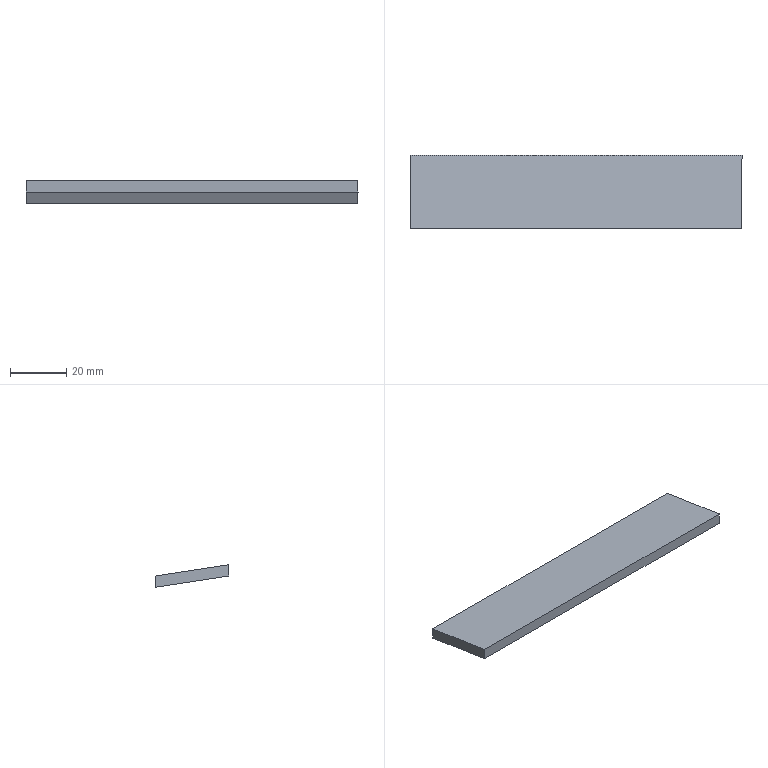Part | SolidWorks | features Blend 1, BlendCut 1, ICE 1 | 1 solid | 6 faces | box 118 x 26 x 8 mm | volume 12272 mm3 | plane 4 | spline 2
STEP:
#1=CARTESIAN_POINT('',(-941.,-26.,-1101.));
#2=VERTEX_POINT('',#1);
#3=CARTESIAN_POINT('',(-941.,-26.,-1105.));
#4=VERTEX_POINT('',#3);
#5=CARTESIAN_POINT('',(-941.,-26.,991.));
#6=DIRECTION('',(0.,0.,-1.));
#7=VECTOR('',#6,1000.);
#8=LINE('',#5,#7);
#9=EDGE_CURVE('',#2,#4,#8,.T.);
#10=ORIENTED_EDGE('',*,*,#9,.F.);
#11=CARTESIAN_POINT('',(-1059.,-26.,-1101.));
#12=VERTEX_POINT('',#11);
#13=CARTESIAN_POINT('',(0.,-26.,-1101.));
#14=DIRECTION('',(-1.,0.,0.));
#15=VECTOR('',#14,1000.);
#16=LINE('',#13,#15);
#17=EDGE_CURVE('',#2,#12,#16,.T.);
#18=ORIENTED_EDGE('',*,*,#17,.T.);
#19=CARTESIAN_POINT('',(-1059.,-26.,-1105.));
#20=VERTEX_POINT('',#19);
#21=CARTESIAN_POINT('',(-1059.,-26.,991.));
#22=DIRECTION('',(0.,0.,1.));
#23=VECTOR('',#22,1000.);
#24=LINE('',#21,#23);
#25=EDGE_CURVE('',#20,#12,#24,.T.);
#26=ORIENTED_EDGE('',*,*,#25,.F.);
#27=CARTESIAN_POINT('',(0.,-26.,-1105.));
#28=DIRECTION('',(1.,0.,0.));
#29=VECTOR('',#28,1000.);
#30=LINE('',#27,#29);
#31=EDGE_CURVE('',#20,#4,#30,.T.);
#32=ORIENTED_EDGE('',*,*,#31,.T.);
#33=EDGE_LOOP('',(#10,#18,#26,#32));
#34=FACE_OUTER_BOUND('',#33,.T.);
#35=CARTESIAN_POINT('',(-1191.,-26.,991.));
#36=DIRECTION('',(0.,1.,0.));
#37=DIRECTION('',(0.,0.,1.));
#38=AXIS2_PLACEMENT_3D('',#35,#36,#37);
#39=PLANE('',#38);
#40=ADVANCED_FACE('',(#34),#39,.F.);
#41=CARTESIAN_POINT('',(-941.,0.,-1105.));
#42=VERTEX_POINT('',#41);
#43=CARTESIAN_POINT('',(-941.,0.,-1109.));
#44=VERTEX_POINT('',#43);
#45=CARTESIAN_POINT('',(-941.,0.,-1109.));
#46=DIRECTION('',(0.,0.,-1.));
#47=VECTOR('',#46,1000.);
#48=LINE('',#45,#47);
#49=EDGE_CURVE('',#42,#44,#48,.T.);
#50=ORIENTED_EDGE('',*,*,#49,.T.);
#51=CARTESIAN_POINT('',(-1059.,0.,-1109.));
#52=VERTEX_POINT('',#51);
#53=CARTESIAN_POINT('',(0.,0.,-1109.));
#54=DIRECTION('',(-1.,0.,0.));
#55=VECTOR('',#54,1000.);
#56=LINE('',#53,#55);
#57=EDGE_CURVE('',#44,#52,#56,.T.);
#58=ORIENTED_EDGE('',*,*,#57,.T.);
#59=CARTESIAN_POINT('',(-1059.,0.,-1105.));
#60=VERTEX_POINT('',#59);
#61=CARTESIAN_POINT('',(-1059.,0.,-1109.));
#62=DIRECTION('',(0.,0.,1.));
#63=VECTOR('',#62,1000.);
#64=LINE('',#61,#63);
#65=EDGE_CURVE('',#52,#60,#64,.T.);
#66=ORIENTED_EDGE('',*,*,#65,.T.);
#67=CARTESIAN_POINT('',(0.,0.,-1105.));
#68=DIRECTION('',(-1.,0.,0.));
#69=VECTOR('',#68,1000.);
#70=LINE('',#67,#69);
#71=EDGE_CURVE('',#42,#60,#70,.T.);
#72=ORIENTED_EDGE('',*,*,#71,.F.);
#73=EDGE_LOOP('',(#50,#58,#66,#72));
#74=FACE_OUTER_BOUND('',#73,.T.);
#75=CARTESIAN_POINT('',(-1191.,0.,991.));
#76=DIRECTION('',(0.,-1.,0.));
#77=DIRECTION('',(0.,0.,-1.));
#78=AXIS2_PLACEMENT_3D('',#75,#76,#77);
#79=PLANE('',#78);
#80=ADVANCED_FACE('',(#74),#79,.F.);
#81=ORIENTED_EDGE('',*,*,#57,.F.);
#82=CARTESIAN_POINT('',(-941.,0.,-1109.));
#83=CARTESIAN_POINT('',(-941.,-2.168,-1108.666));
#84=CARTESIAN_POINT('',(-941.,-4.336,-1108.333));
#85=CARTESIAN_POINT('',(-941.,-6.504,-1107.999));
#86=CARTESIAN_POINT('',(-941.,-8.672,-1107.666));
#87=CARTESIAN_POINT('',(-941.,-10.84,-1107.332));
#88=CARTESIAN_POINT('',(-941.,-13.008,-1106.999));
#89=CARTESIAN_POINT('',(-941.,-17.338,-1106.333));
#90=CARTESIAN_POINT('',(-941.,-21.669,-1105.666));
#91=CARTESIAN_POINT('',(-941.,-26.,-1105.));
#92=B_SPLINE_CURVE_WITH_KNOTS('',3,(#82,#83,#84,#85,#86,#87,#88,#89,#90,#91),.UNSPECIFIED.,.F.,.F.,(4,3,3,4),(0.,0.00658,0.01316,0.02631),.UNSPECIFIED.);
#93=EDGE_CURVE('',#44,#4,#92,.T.);
#94=ORIENTED_EDGE('',*,*,#93,.T.);
#95=ORIENTED_EDGE('',*,*,#31,.F.);
#96=CARTESIAN_POINT('',(-1059.,-26.,-1105.));
#97=CARTESIAN_POINT('',(-1059.,-23.832,-1105.334));
#98=CARTESIAN_POINT('',(-1059.,-21.664,-1105.667));
#99=CARTESIAN_POINT('',(-1059.,-19.496,-1106.001));
#100=CARTESIAN_POINT('',(-1059.,-17.328,-1106.334));
#101=CARTESIAN_POINT('',(-1059.,-15.16,-1106.668));
#102=CARTESIAN_POINT('',(-1059.,-12.992,-1107.001));
#103=CARTESIAN_POINT('',(-1059.,-8.662,-1107.667));
#104=CARTESIAN_POINT('',(-1059.,-4.331,-1108.334));
#105=CARTESIAN_POINT('',(-1059.,0.,-1109.));
#106=B_SPLINE_CURVE_WITH_KNOTS('',3,(#96,#97,#98,#99,#100,#101,#102,#103,#104,#105),.UNSPECIFIED.,.F.,.F.,(4,3,3,4),(0.,0.00658,0.01316,0.02631),.UNSPECIFIED.);
#107=EDGE_CURVE('',#20,#52,#106,.T.);
#108=ORIENTED_EDGE('',*,*,#107,.T.);
#109=EDGE_LOOP('',(#81,#94,#95,#108));
#110=FACE_OUTER_BOUND('',#109,.T.);
#111=CARTESIAN_POINT('',(-1309.,0.,991.));
#112=CARTESIAN_POINT('',(-1305.,-26.,991.));
#113=CARTESIAN_POINT('',(-1309.,0.,825.593));
#114=CARTESIAN_POINT('',(-1305.,-26.,826.073));
#115=CARTESIAN_POINT('',(-1309.,0.,495.141));
#116=CARTESIAN_POINT('',(-1305.,-26.,495.86));
#117=CARTESIAN_POINT('',(-1309.,0.,0.));
#118=CARTESIAN_POINT('',(-1305.,-26.,0.));
#119=CARTESIAN_POINT('',(-1309.,0.,-495.141));
#120=CARTESIAN_POINT('',(-1305.,-26.,-495.86));
#121=CARTESIAN_POINT('',(-1309.,0.,-825.593));
#122=CARTESIAN_POINT('',(-1305.,-26.,-826.073));
#123=CARTESIAN_POINT('',(-1309.,0.,-998.603));
#124=CARTESIAN_POINT('',(-1305.,-26.,-998.581));
#125=CARTESIAN_POINT('',(-1307.525,0.,-1013.896));
#126=CARTESIAN_POINT('',(-1303.485,-26.,-1013.65));
#127=CARTESIAN_POINT('',(-1300.841,0.,-1036.165));
#128=CARTESIAN_POINT('',(-1296.885,-26.,-1035.179));
#129=CARTESIAN_POINT('',(-1289.866,0.,-1056.819));
#130=CARTESIAN_POINT('',(-1286.285,-26.,-1054.896));
#131=CARTESIAN_POINT('',(-1275.,0.,-1074.971));
#132=CARTESIAN_POINT('',(-1272.108,-26.,-1072.135));
#133=CARTESIAN_POINT('',(-1256.851,0.,-1089.845));
#134=CARTESIAN_POINT('',(-1254.866,-26.,-1086.305));
#135=CARTESIAN_POINT('',(-1236.193,0.,-1100.83));
#136=CARTESIAN_POINT('',(-1235.152,-26.,-1096.895));
#137=CARTESIAN_POINT('',(-1213.914,0.,-1107.523));
#138=CARTESIAN_POINT('',(-1213.633,-26.,-1103.487));
#139=CARTESIAN_POINT('',(-1198.609,0.,-1109.));
#140=CARTESIAN_POINT('',(-1198.575,-26.,-1105.));
#141=CARTESIAN_POINT('',(-1091.523,0.,-1109.));
#142=CARTESIAN_POINT('',(-1091.977,-26.,-1105.));
#143=CARTESIAN_POINT('',(-892.796,0.,-1109.));
#144=CARTESIAN_POINT('',(-893.704,-26.,-1105.));
#145=CARTESIAN_POINT('',(-595.132,0.,-1109.));
#146=CARTESIAN_POINT('',(-595.87,-26.,-1105.));
#147=CARTESIAN_POINT('',(-297.637,0.,-1109.));
#148=CARTESIAN_POINT('',(-297.864,-26.,-1105.));
#149=CARTESIAN_POINT('',(-99.25,0.,-1109.));
#150=CARTESIAN_POINT('',(-99.25,-26.,-1105.));
#151=CARTESIAN_POINT('',(99.25,0.,-1109.));
#152=CARTESIAN_POINT('',(99.25,-26.,-1105.));
#153=CARTESIAN_POINT('',(297.637,0.,-1109.));
#154=CARTESIAN_POINT('',(297.864,-26.,-1105.));
#155=CARTESIAN_POINT('',(595.132,0.,-1109.));
#156=CARTESIAN_POINT('',(595.87,-26.,-1105.));
#157=CARTESIAN_POINT('',(892.796,0.,-1109.));
#158=CARTESIAN_POINT('',(893.704,-26.,-1105.));
#159=CARTESIAN_POINT('',(1091.523,0.,-1109.));
#160=CARTESIAN_POINT('',(1091.977,-26.,-1105.));
#161=CARTESIAN_POINT('',(1198.609,0.,-1109.));
#162=CARTESIAN_POINT('',(1198.575,-26.,-1105.));
#163=CARTESIAN_POINT('',(1213.914,0.,-1107.523));
#164=CARTESIAN_POINT('',(1213.633,-26.,-1103.487));
#165=CARTESIAN_POINT('',(1236.193,0.,-1100.83));
#166=CARTESIAN_POINT('',(1235.152,-26.,-1096.895));
#167=CARTESIAN_POINT('',(1256.851,0.,-1089.845));
#168=CARTESIAN_POINT('',(1254.866,-26.,-1086.305));
#169=CARTESIAN_POINT('',(1275.,0.,-1074.971));
#170=CARTESIAN_POINT('',(1272.108,-26.,-1072.135));
#171=CARTESIAN_POINT('',(1289.866,0.,-1056.819));
#172=CARTESIAN_POINT('',(1286.285,-26.,-1054.896));
#173=CARTESIAN_POINT('',(1300.841,0.,-1036.165));
#174=CARTESIAN_POINT('',(1296.885,-26.,-1035.179));
#175=CARTESIAN_POINT('',(1307.525,0.,-1013.896));
#176=CARTESIAN_POINT('',(1303.485,-26.,-1013.65));
#177=CARTESIAN_POINT('',(1309.,0.,-998.603));
#178=CARTESIAN_POINT('',(1305.,-26.,-998.581));
#179=CARTESIAN_POINT('',(1309.,0.,-825.593));
#180=CARTESIAN_POINT('',(1305.,-26.,-826.073));
#181=CARTESIAN_POINT('',(1309.,0.,-495.141));
#182=CARTESIAN_POINT('',(1305.,-26.,-495.86));
#183=CARTESIAN_POINT('',(1309.,0.,0.));
#184=CARTESIAN_POINT('',(1305.,-26.,0.));
#185=CARTESIAN_POINT('',(1309.,0.,495.141));
#186=CARTESIAN_POINT('',(1305.,-26.,495.86));
#187=CARTESIAN_POINT('',(1309.,0.,825.593));
#188=CARTESIAN_POINT('',(1305.,-26.,826.073));
#189=CARTESIAN_POINT('',(1309.,0.,998.603));
#190=CARTESIAN_POINT('',(1305.,-26.,998.581));
#191=CARTESIAN_POINT('',(1307.525,0.,1013.896));
#192=CARTESIAN_POINT('',(1303.485,-26.,1013.65));
#193=CARTESIAN_POINT('',(1300.841,0.,1036.165));
#194=CARTESIAN_POINT('',(1296.885,-26.,1035.179));
#195=CARTESIAN_POINT('',(1289.866,0.,1056.819));
#196=CARTESIAN_POINT('',(1286.285,-26.,1054.896));
#197=CARTESIAN_POINT('',(1275.,0.,1074.971));
#198=CARTESIAN_POINT('',(1272.108,-26.,1072.135));
#199=CARTESIAN_POINT('',(1256.851,0.,1089.845));
#200=CARTESIAN_POINT('',(1254.866,-26.,1086.305));
#201=CARTESIAN_POINT('',(1236.193,0.,1100.83));
#202=CARTESIAN_POINT('',(1235.152,-26.,1096.895));
#203=CARTESIAN_POINT('',(1213.914,0.,1107.523));
#204=CARTESIAN_POINT('',(1213.633,-26.,1103.487));
#205=CARTESIAN_POINT('',(1198.609,0.,1109.));
#206=CARTESIAN_POINT('',(1198.575,-26.,1105.));
#207=CARTESIAN_POINT('',(1091.523,0.,1109.));
#208=CARTESIAN_POINT('',(1091.977,-26.,1105.));
#209=CARTESIAN_POINT('',(892.796,0.,1109.));
#210=CARTESIAN_POINT('',(893.704,-26.,1105.));
#211=CARTESIAN_POINT('',(595.132,0.,1109.));
#212=CARTESIAN_POINT('',(595.87,-26.,1105.));
#213=CARTESIAN_POINT('',(297.637,0.,1109.));
#214=CARTESIAN_POINT('',(297.864,-26.,1105.));
#215=CARTESIAN_POINT('',(99.25,0.,1109.));
#216=CARTESIAN_POINT('',(99.25,-26.,1105.));
#217=CARTESIAN_POINT('',(-99.25,0.,1109.));
#218=CARTESIAN_POINT('',(-99.25,-26.,1105.));
#219=CARTESIAN_POINT('',(-297.637,0.,1109.));
#220=CARTESIAN_POINT('',(-297.864,-26.,1105.));
#221=CARTESIAN_POINT('',(-595.132,0.,1109.));
#222=CARTESIAN_POINT('',(-595.87,-26.,1105.));
#223=CARTESIAN_POINT('',(-892.796,0.,1109.));
#224=CARTESIAN_POINT('',(-893.704,-26.,1105.));
#225=CARTESIAN_POINT('',(-1091.523,0.,1109.));
#226=CARTESIAN_POINT('',(-1091.977,-26.,1105.));
#227=CARTESIAN_POINT('',(-1198.609,0.,1109.));
#228=CARTESIAN_POINT('',(-1198.575,-26.,1105.));
#229=CARTESIAN_POINT('',(-1213.914,0.,1107.523));
#230=CARTESIAN_POINT('',(-1213.633,-26.,1103.487));
#231=CARTESIAN_POINT('',(-1236.193,0.,1100.83));
#232=CARTESIAN_POINT('',(-1235.152,-26.,1096.895));
#233=CARTESIAN_POINT('',(-1256.851,0.,1089.845));
#234=CARTESIAN_POINT('',(-1254.866,-26.,1086.305));
#235=CARTESIAN_POINT('',(-1275.,0.,1074.971));
#236=CARTESIAN_POINT('',(-1272.108,-26.,1072.135));
#237=CARTESIAN_POINT('',(-1289.866,0.,1056.819));
#238=CARTESIAN_POINT('',(-1286.285,-26.,1054.896));
#239=CARTESIAN_POINT('',(-1300.841,0.,1036.165));
#240=CARTESIAN_POINT('',(-1296.885,-26.,1035.179));
#241=CARTESIAN_POINT('',(-1307.525,0.,1013.896));
#242=CARTESIAN_POINT('',(-1303.485,-26.,1013.65));
#243=CARTESIAN_POINT('',(-1309.,0.,998.603));
#244=CARTESIAN_POINT('',(-1305.,-26.,998.581));
#245=CARTESIAN_POINT('',(-1309.,0.,991.));
#246=CARTESIAN_POINT('',(-1305.,-26.,991.));
#247=B_SPLINE_SURFACE_WITH_KNOTS('',3,1,((#111,#112),(#113,#114),(#115,#116),(#117,#118),(#119,#120),(#121,#122),(#123,#124),(#125,#126),(#127,#128),(#129,#130),(#131,#132),(#133,#134),(#135,#136),(#137,#138),(#139,#140),(#141,#142),(#143,#144),(#145,#146),(#147,#148),(#149,#150),(#151,#152),(#153,#154),(#155,#156),(#157,#158),(#159,#160),(#161,#162),(#163,#164),(#165,#166),(#167,#168),(#169,#170),(#171,#172),(#173,#174),(#175,#176),(#177,#178),(#179,#180),(#181,#182),(#183,#184),(#185,#186),(#187,#188),(#189,#190),(#191,#192),(#193,#194),(#195,#196),(#197,#198),(#199,#200),(#201,#202),(#203,#204),(#205,#206),(#207,#208),(#209,#210),(#211,#212),(#213,#214),(#215,#216),(#217,#218),(#219,#220),(#221,#222),(#223,#224),(#225,#226),(#227,#228),(#229,#230),(#231,#232),(#233,#234),(#235,#236),(#237,#238),(#239,#240),(#241,#242),(#243,#244),(#245,#246)),.UNSPECIFIED.,.T.,.F.,.F.,(4,1,1,1,2,1,1,1,1,1,1,1,2,1,1,1,2,1,1,1,2,1,1,1,1,1,1,1,2,1,1,1,2,1,1,1,1,1,1,1,2,1,1,1,2,1,1,1,2,1,1,1,1,1,1,1,4),(2,2),(0.,0.0524,0.1048,0.1572,0.2096,0.212,0.2144,0.2168,0.2192,0.2216,0.224,0.2264,0.2289,0.2603,0.2918,0.3233,0.3548,0.3863,0.4178,0.4492,0.4807,0.4831,0.4855,0.488,0.4904,0.4928,0.4952,0.4976,0.5,0.5524,0.6048,0.6572,0.7096,0.712,0.7144,0.7168,0.7192,0.7216,0.724,0.7264,0.7289,0.7603,0.7918,0.8233,0.8548,0.8863,0.9178,0.9492,0.9807,0.9831,0.9855,0.988,0.9904,0.9928,0.9952,0.9976,1.),(0.,1.),.UNSPECIFIED.);
#248=ADVANCED_FACE('',(#110),#247,.T.);
#249=CARTESIAN_POINT('',(-941.,0.,-1105.));
#250=CARTESIAN_POINT('',(-941.,-2.168,-1104.666));
#251=CARTESIAN_POINT('',(-941.,-4.336,-1104.333));
#252=CARTESIAN_POINT('',(-941.,-6.504,-1103.999));
#253=CARTESIAN_POINT('',(-941.,-8.672,-1103.666));
#254=CARTESIAN_POINT('',(-941.,-10.84,-1103.332));
#255=CARTESIAN_POINT('',(-941.,-13.008,-1102.999));
#256=CARTESIAN_POINT('',(-941.,-17.339,-1102.333));
#257=CARTESIAN_POINT('',(-941.,-21.669,-1101.666));
#258=CARTESIAN_POINT('',(-941.,-26.,-1101.));
#259=B_SPLINE_CURVE_WITH_KNOTS('',3,(#249,#250,#251,#252,#253,#254,#255,#256,#257,#258),.UNSPECIFIED.,.F.,.F.,(4,3,3,4),(0.,0.00658,0.01316,0.02631),.UNSPECIFIED.);
#260=EDGE_CURVE('',#42,#2,#259,.T.);
#261=ORIENTED_EDGE('',*,*,#260,.F.);
#262=ORIENTED_EDGE('',*,*,#71,.T.);
#263=CARTESIAN_POINT('',(-1059.,-26.,-1101.));
#264=CARTESIAN_POINT('',(-1059.,-23.832,-1101.334));
#265=CARTESIAN_POINT('',(-1059.,-21.664,-1101.667));
#266=CARTESIAN_POINT('',(-1059.,-19.496,-1102.001));
#267=CARTESIAN_POINT('',(-1059.,-17.328,-1102.334));
#268=CARTESIAN_POINT('',(-1059.,-15.16,-1102.668));
#269=CARTESIAN_POINT('',(-1059.,-12.992,-1103.001));
#270=CARTESIAN_POINT('',(-1059.,-8.661,-1103.667));
#271=CARTESIAN_POINT('',(-1059.,-4.331,-1104.334));
#272=CARTESIAN_POINT('',(-1059.,0.,-1105.));
#273=B_SPLINE_CURVE_WITH_KNOTS('',3,(#263,#264,#265,#266,#267,#268,#269,#270,#271,#272),.UNSPECIFIED.,.F.,.F.,(4,3,3,4),(0.,0.00658,0.01316,0.02631),.UNSPECIFIED.);
#274=EDGE_CURVE('',#12,#60,#273,.T.);
#275=ORIENTED_EDGE('',*,*,#274,.F.);
#276=ORIENTED_EDGE('',*,*,#17,.F.);
#277=EDGE_LOOP('',(#261,#262,#275,#276));
#278=FACE_OUTER_BOUND('',#277,.T.);
#279=CARTESIAN_POINT('',(-1305.,0.,991.));
#280=CARTESIAN_POINT('',(-1301.,-26.,991.));
#281=CARTESIAN_POINT('',(-1305.,0.,825.593));
#282=CARTESIAN_POINT('',(-1301.,-26.,826.073));
#283=CARTESIAN_POINT('',(-1305.,0.,495.14));
#284=CARTESIAN_POINT('',(-1301.,-26.,495.861));
#285=CARTESIAN_POINT('',(-1305.,0.,0.));
#286=CARTESIAN_POINT('',(-1301.,-26.,0.));
#287=CARTESIAN_POINT('',(-1305.,0.,-495.14));
#288=CARTESIAN_POINT('',(-1301.,-26.,-495.861));
#289=CARTESIAN_POINT('',(-1305.,0.,-825.593));
#290=CARTESIAN_POINT('',(-1301.,-26.,-826.073));
#291=CARTESIAN_POINT('',(-1305.,0.,-998.341));
#292=CARTESIAN_POINT('',(-1301.,-26.,-998.32));
#293=CARTESIAN_POINT('',(-1303.577,0.,-1013.11));
#294=CARTESIAN_POINT('',(-1299.536,-26.,-1012.866));
#295=CARTESIAN_POINT('',(-1297.122,0.,-1034.623));
#296=CARTESIAN_POINT('',(-1293.165,-26.,-1033.638));
#297=CARTESIAN_POINT('',(-1286.518,0.,-1054.583));
#298=CARTESIAN_POINT('',(-1282.938,-26.,-1052.659));
#299=CARTESIAN_POINT('',(-1272.153,0.,-1072.125));
#300=CARTESIAN_POINT('',(-1269.262,-26.,-1069.288));
#301=CARTESIAN_POINT('',(-1254.614,0.,-1086.498));
#302=CARTESIAN_POINT('',(-1252.63,-26.,-1082.957));
#303=CARTESIAN_POINT('',(-1234.651,0.,-1097.111));
#304=CARTESIAN_POINT('',(-1233.612,-26.,-1093.175));
#305=CARTESIAN_POINT('',(-1213.127,0.,-1103.574));
#306=CARTESIAN_POINT('',(-1212.849,-26.,-1099.539));
#307=CARTESIAN_POINT('',(-1198.347,0.,-1105.));
#308=CARTESIAN_POINT('',(-1198.313,-26.,-1101.));
#309=CARTESIAN_POINT('',(-1091.522,0.,-1105.));
#310=CARTESIAN_POINT('',(-1091.978,-26.,-1101.));
#311=CARTESIAN_POINT('',(-892.794,0.,-1105.));
#312=CARTESIAN_POINT('',(-893.707,-26.,-1101.));
#313=CARTESIAN_POINT('',(-595.13,0.,-1105.));
#314=CARTESIAN_POINT('',(-595.871,-26.,-1101.));
#315=CARTESIAN_POINT('',(-297.636,0.,-1105.));
#316=CARTESIAN_POINT('',(-297.864,-26.,-1101.));
#317=CARTESIAN_POINT('',(-99.25,0.,-1105.));
#318=CARTESIAN_POINT('',(-99.25,-26.,-1101.));
#319=CARTESIAN_POINT('',(99.25,0.,-1105.));
#320=CARTESIAN_POINT('',(99.25,-26.,-1101.));
#321=CARTESIAN_POINT('',(297.636,0.,-1105.));
#322=CARTESIAN_POINT('',(297.864,-26.,-1101.));
#323=CARTESIAN_POINT('',(595.13,0.,-1105.));
#324=CARTESIAN_POINT('',(595.871,-26.,-1101.));
#325=CARTESIAN_POINT('',(892.794,0.,-1105.));
#326=CARTESIAN_POINT('',(893.707,-26.,-1101.));
#327=CARTESIAN_POINT('',(1091.522,0.,-1105.));
#328=CARTESIAN_POINT('',(1091.978,-26.,-1101.));
#329=CARTESIAN_POINT('',(1198.347,0.,-1105.));
#330=CARTESIAN_POINT('',(1198.313,-26.,-1101.));
#331=CARTESIAN_POINT('',(1213.127,0.,-1103.574));
#332=CARTESIAN_POINT('',(1212.849,-26.,-1099.539));
#333=CARTESIAN_POINT('',(1234.651,0.,-1097.111));
#334=CARTESIAN_POINT('',(1233.612,-26.,-1093.175));
#335=CARTESIAN_POINT('',(1254.614,0.,-1086.498));
#336=CARTESIAN_POINT('',(1252.63,-26.,-1082.957));
#337=CARTESIAN_POINT('',(1272.153,0.,-1072.125));
#338=CARTESIAN_POINT('',(1269.262,-26.,-1069.288));
#339=CARTESIAN_POINT('',(1286.518,0.,-1054.583));
#340=CARTESIAN_POINT('',(1282.938,-26.,-1052.659));
#341=CARTESIAN_POINT('',(1297.122,0.,-1034.623));
#342=CARTESIAN_POINT('',(1293.165,-26.,-1033.638));
#343=CARTESIAN_POINT('',(1303.577,0.,-1013.11));
#344=CARTESIAN_POINT('',(1299.536,-26.,-1012.866));
#345=CARTESIAN_POINT('',(1305.,0.,-998.341));
#346=CARTESIAN_POINT('',(1301.,-26.,-998.32));
#347=CARTESIAN_POINT('',(1305.,0.,-825.593));
#348=CARTESIAN_POINT('',(1301.,-26.,-826.073));
#349=CARTESIAN_POINT('',(1305.,0.,-495.14));
#350=CARTESIAN_POINT('',(1301.,-26.,-495.861));
#351=CARTESIAN_POINT('',(1305.,0.,0.));
#352=CARTESIAN_POINT('',(1301.,-26.,0.));
#353=CARTESIAN_POINT('',(1305.,0.,495.14));
#354=CARTESIAN_POINT('',(1301.,-26.,495.861));
#355=CARTESIAN_POINT('',(1305.,0.,825.593));
#356=CARTESIAN_POINT('',(1301.,-26.,826.073));
#357=CARTESIAN_POINT('',(1305.,0.,998.341));
#358=CARTESIAN_POINT('',(1301.,-26.,998.32));
#359=CARTESIAN_POINT('',(1303.577,0.,1013.11));
#360=CARTESIAN_POINT('',(1299.536,-26.,1012.866));
#361=CARTESIAN_POINT('',(1297.122,0.,1034.623));
#362=CARTESIAN_POINT('',(1293.165,-26.,1033.638));
#363=CARTESIAN_POINT('',(1286.518,0.,1054.583));
#364=CARTESIAN_POINT('',(1282.938,-26.,1052.659));
#365=CARTESIAN_POINT('',(1272.153,0.,1072.125));
#366=CARTESIAN_POINT('',(1269.262,-26.,1069.288));
#367=CARTESIAN_POINT('',(1254.614,0.,1086.498));
#368=CARTESIAN_POINT('',(1252.63,-26.,1082.957));
#369=CARTESIAN_POINT('',(1234.651,0.,1097.111));
#370=CARTESIAN_POINT('',(1233.612,-26.,1093.175));
#371=CARTESIAN_POINT('',(1213.127,0.,1103.574));
#372=CARTESIAN_POINT('',(1212.849,-26.,1099.539));
#373=CARTESIAN_POINT('',(1198.347,0.,1105.));
#374=CARTESIAN_POINT('',(1198.313,-26.,1101.));
#375=CARTESIAN_POINT('',(1091.522,0.,1105.));
#376=CARTESIAN_POINT('',(1091.978,-26.,1101.));
#377=CARTESIAN_POINT('',(892.794,0.,1105.));
#378=CARTESIAN_POINT('',(893.707,-26.,1101.));
#379=CARTESIAN_POINT('',(595.13,0.,1105.));
#380=CARTESIAN_POINT('',(595.871,-26.,1101.));
#381=CARTESIAN_POINT('',(297.636,0.,1105.));
#382=CARTESIAN_POINT('',(297.864,-26.,1101.));
#383=CARTESIAN_POINT('',(99.25,0.,1105.));
#384=CARTESIAN_POINT('',(99.25,-26.,1101.));
#385=CARTESIAN_POINT('',(-99.25,0.,1105.));
#386=CARTESIAN_POINT('',(-99.25,-26.,1101.));
#387=CARTESIAN_POINT('',(-297.636,0.,1105.));
#388=CARTESIAN_POINT('',(-297.864,-26.,1101.));
#389=CARTESIAN_POINT('',(-595.13,0.,1105.));
#390=CARTESIAN_POINT('',(-595.871,-26.,1101.));
#391=CARTESIAN_POINT('',(-892.794,0.,1105.));
#392=CARTESIAN_POINT('',(-893.707,-26.,1101.));
#393=CARTESIAN_POINT('',(-1091.522,0.,1105.));
#394=CARTESIAN_POINT('',(-1091.978,-26.,1101.));
#395=CARTESIAN_POINT('',(-1198.347,0.,1105.));
#396=CARTESIAN_POINT('',(-1198.313,-26.,1101.));
#397=CARTESIAN_POINT('',(-1213.127,0.,1103.574));
#398=CARTESIAN_POINT('',(-1212.849,-26.,1099.539));
#399=CARTESIAN_POINT('',(-1234.651,0.,1097.111));
#400=CARTESIAN_POINT('',(-1233.612,-26.,1093.175));
#401=CARTESIAN_POINT('',(-1254.614,0.,1086.498));
#402=CARTESIAN_POINT('',(-1252.63,-26.,1082.957));
#403=CARTESIAN_POINT('',(-1272.153,0.,1072.125));
#404=CARTESIAN_POINT('',(-1269.262,-26.,1069.288));
#405=CARTESIAN_POINT('',(-1286.518,0.,1054.583));
#406=CARTESIAN_POINT('',(-1282.938,-26.,1052.659));
#407=CARTESIAN_POINT('',(-1297.122,0.,1034.623));
#408=CARTESIAN_POINT('',(-1293.165,-26.,1033.638));
#409=CARTESIAN_POINT('',(-1303.577,0.,1013.11));
#410=CARTESIAN_POINT('',(-1299.536,-26.,1012.866));
#411=CARTESIAN_POINT('',(-1305.,0.,998.341));
#412=CARTESIAN_POINT('',(-1301.,-26.,998.32));
#413=CARTESIAN_POINT('',(-1305.,0.,991.));
#414=CARTESIAN_POINT('',(-1301.,-26.,991.));
#415=B_SPLINE_SURFACE_WITH_KNOTS('',3,1,((#279,#280),(#281,#282),(#283,#284),(#285,#286),(#287,#288),(#289,#290),(#291,#292),(#293,#294),(#295,#296),(#297,#298),(#299,#300),(#301,#302),(#303,#304),(#305,#306),(#307,#308),(#309,#310),(#311,#312),(#313,#314),(#315,#316),(#317,#318),(#319,#320),(#321,#322),(#323,#324),(#325,#326),(#327,#328),(#329,#330),(#331,#332),(#333,#334),(#335,#336),(#337,#338),(#339,#340),(#341,#342),(#343,#344),(#345,#346),(#347,#348),(#349,#350),(#351,#352),(#353,#354),(#355,#356),(#357,#358),(#359,#360),(#361,#362),(#363,#364),(#365,#366),(#367,#368),(#369,#370),(#371,#372),(#373,#374),(#375,#376),(#377,#378),(#379,#380),(#381,#382),(#383,#384),(#385,#386),(#387,#388),(#389,#390),(#391,#392),(#393,#394),(#395,#396),(#397,#398),(#399,#400),(#401,#402),(#403,#404),(#405,#406),(#407,#408),(#409,#410),(#411,#412),(#413,#414)),.UNSPECIFIED.,.T.,.F.,.F.,(4,1,1,1,2,1,1,1,1,1,1,1,2,1,1,1,2,1,1,1,2,1,1,1,1,1,1,1,2,1,1,1,2,1,1,1,1,1,1,1,2,1,1,1,2,1,1,1,2,1,1,1,1,1,1,1,4),(2,2),(0.,0.05254,0.1051,0.1576,0.2101,0.2125,0.2148,0.2171,0.2195,0.2218,0.2241,0.2265,0.2288,0.2604,0.2919,0.3235,0.3551,0.3866,0.4182,0.4498,0.4813,0.4837,0.486,0.4883,0.4907,0.493,0.4953,0.4977,0.5,0.5525,0.6051,0.6576,0.7101,0.7125,0.7148,0.7171,0.7195,0.7218,0.7241,0.7265,0.7288,0.7604,0.7919,0.8235,0.8551,0.8866,0.9182,0.9498,0.9813,0.9837,0.986,0.9883,0.9907,0.993,0.9953,0.9977,1.),(0.,1.),.UNSPECIFIED.);
#416=ADVANCED_FACE('',(#278),#415,.F.);
#417=ORIENTED_EDGE('',*,*,#25,.T.);
#418=ORIENTED_EDGE('',*,*,#274,.T.);
#419=ORIENTED_EDGE('',*,*,#65,.F.);
#420=ORIENTED_EDGE('',*,*,#107,.F.);
#421=EDGE_LOOP('',(#417,#418,#419,#420));
#422=FACE_OUTER_BOUND('',#421,.T.);
#423=CARTESIAN_POINT('',(-1059.,-26.005,-1109.));
#424=DIRECTION('',(-1.,0.,0.));
#425=DIRECTION('',(0.,0.,1.));
#426=AXIS2_PLACEMENT_3D('',#423,#424,#425);
#427=PLANE('',#426);
#428=ADVANCED_FACE('',(#422),#427,.T.);
#429=ORIENTED_EDGE('',*,*,#49,.F.);
#430=ORIENTED_EDGE('',*,*,#260,.T.);
#431=ORIENTED_EDGE('',*,*,#9,.T.);
#432=ORIENTED_EDGE('',*,*,#93,.F.);
#433=EDGE_LOOP('',(#429,#430,#431,#432));
#434=FACE_OUTER_BOUND('',#433,.T.);
#435=CARTESIAN_POINT('',(-941.,-26.005,-1109.));
#436=DIRECTION('',(1.,0.,0.));
#437=DIRECTION('',(0.,0.,-1.));
#438=AXIS2_PLACEMENT_3D('',#435,#436,#437);
#439=PLANE('',#438);
#440=ADVANCED_FACE('',(#434),#439,.T.);
#441=CLOSED_SHELL('',(#40,#80,#248,#416,#428,#440));
#442=MANIFOLD_SOLID_BREP('',#441);
#443=CARTESIAN_POINT('',(0.,0.,0.));
#444=DIRECTION('',(0.,0.,1.));
#445=DIRECTION('',(1.,0.,0.));
#446=AXIS2_PLACEMENT_3D('',#443,#444,#445);
#447=(LENGTH_UNIT()NAMED_UNIT(*)SI_UNIT(.MILLI.,.METRE.));
#448=UNCERTAINTY_MEASURE_WITH_UNIT(LENGTH_MEASURE(0.00001),#447,'','');
#449=(NAMED_UNIT(*)PLANE_ANGLE_UNIT()SI_UNIT($,.RADIAN.));
#450=(NAMED_UNIT(*)SI_UNIT($,.STERADIAN.)SOLID_ANGLE_UNIT());
#451=(GEOMETRIC_REPRESENTATION_CONTEXT(3)GLOBAL_UNCERTAINTY_ASSIGNED_CONTEXT((#448))GLOBAL_UNIT_ASSIGNED_CONTEXT((#447,#449,#450))REPRESENTATION_CONTEXT('',''));
#452=ADVANCED_BREP_SHAPE_REPRESENTATION('',(#442,#446),#451);